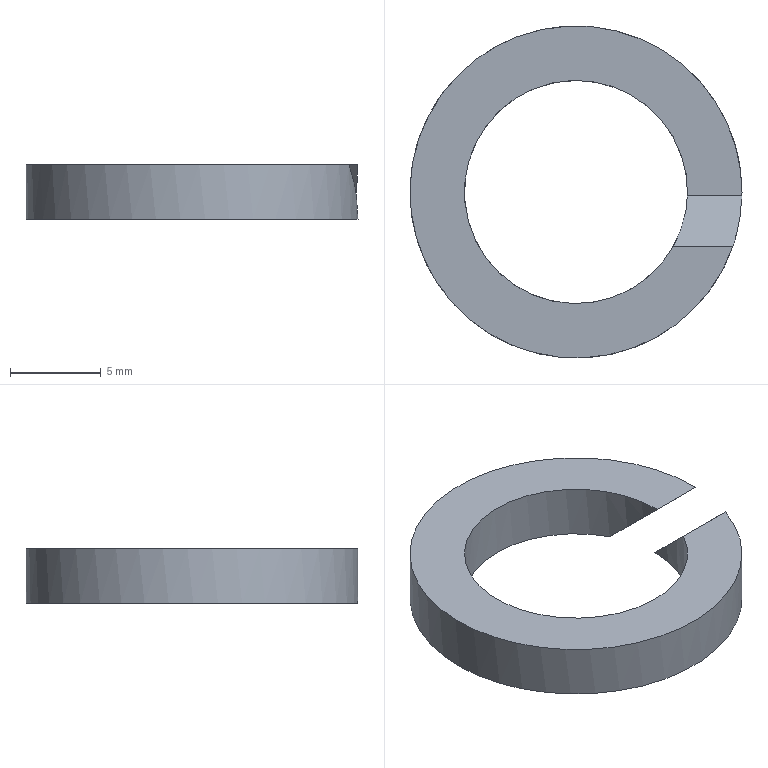Part | NX | features DATUM_CSYS 3, EXTRUDE 2, SKETCH 2 | 1 solid | 6 faces | box 18.3 x 18.3 x 3 mm | volume 406.803 mm3 | plane 4 | cylinder 2 | commonest cylinder face diameters 12.3 x1 18.3 x1
STEP:
#1=CARTESIAN_POINT('',(9.148,-0.1716,0.));
#2=VERTEX_POINT('',#1);
#3=CARTESIAN_POINT('',(8.644,-3.,0.));
#4=VERTEX_POINT('',#3);
#5=CARTESIAN_POINT('',(0.,0.,0.));
#6=DIRECTION('',(0.,0.,1.));
#7=DIRECTION('',(1.,0.,0.));
#8=AXIS2_PLACEMENT_3D('',#5,#6,#7);
#9=CIRCLE('',#8,9.15);
#10=EDGE_CURVE('',#2,#4,#9,.T.);
#11=ORIENTED_EDGE('',*,*,#10,.T.);
#12=CARTESIAN_POINT('',(5.369,-3.,0.));
#13=VERTEX_POINT('',#12);
#14=CARTESIAN_POINT('',(16.9,-3.,0.));
#15=DIRECTION('',(-1.,0.,0.));
#16=VECTOR('',#15,1000.);
#17=LINE('',#14,#16);
#18=EDGE_CURVE('',#4,#13,#17,.T.);
#19=ORIENTED_EDGE('',*,*,#18,.T.);
#20=CARTESIAN_POINT('',(6.148,-0.1716,0.));
#21=VERTEX_POINT('',#20);
#22=CARTESIAN_POINT('',(0.,0.,0.));
#23=DIRECTION('',(0.,0.,1.));
#24=DIRECTION('',(1.,0.,0.));
#25=AXIS2_PLACEMENT_3D('',#22,#23,#24);
#26=CIRCLE('',#25,6.15);
#27=EDGE_CURVE('',#21,#13,#26,.T.);
#28=ORIENTED_EDGE('',*,*,#27,.F.);
#29=CARTESIAN_POINT('',(16.9,-0.1716,0.));
#30=DIRECTION('',(-1.,0.,0.));
#31=VECTOR('',#30,1000.);
#32=LINE('',#29,#31);
#33=EDGE_CURVE('',#2,#21,#32,.T.);
#34=ORIENTED_EDGE('',*,*,#33,.F.);
#35=EDGE_LOOP('',(#11,#19,#28,#34));
#36=FACE_BOUND('',#35,.T.);
#37=CARTESIAN_POINT('',(0.,0.,0.));
#38=DIRECTION('',(0.,0.,1.));
#39=DIRECTION('',(1.,0.,0.));
#40=AXIS2_PLACEMENT_3D('',#37,#38,#39);
#41=PLANE('',#40);
#42=ADVANCED_FACE('',(#36),#41,.T.);
#43=CARTESIAN_POINT('',(8.702,2.828,-3.));
#44=VERTEX_POINT('',#43);
#45=CARTESIAN_POINT('',(0.,0.,-0.1716));
#46=DIRECTION('',(0.,0.7071,0.7071));
#47=DIRECTION('',(0.,-0.7071,0.7071));
#48=AXIS2_PLACEMENT_3D('',#45,#46,#47);
#49=ELLIPSE('',#48,12.94,9.15);
#50=EDGE_CURVE('',#44,#2,#49,.F.);
#51=ORIENTED_EDGE('',*,*,#50,.F.);
#52=CARTESIAN_POINT('',(9.15,0.,-3.));
#53=VERTEX_POINT('',#52);
#54=CARTESIAN_POINT('',(0.,0.,-3.));
#55=DIRECTION('',(0.,0.,1.));
#56=DIRECTION('',(1.,0.,0.));
#57=AXIS2_PLACEMENT_3D('',#54,#55,#56);
#58=CIRCLE('',#57,9.15);
#59=EDGE_CURVE('',#44,#53,#58,.T.);
#60=ORIENTED_EDGE('',*,*,#59,.T.);
#61=CARTESIAN_POINT('',(0.,0.,-3.));
#62=DIRECTION('',(0.,-0.7071,-0.7071));
#63=DIRECTION('',(0.,-0.7071,0.7071));
#64=AXIS2_PLACEMENT_3D('',#61,#62,#63);
#65=ELLIPSE('',#64,12.94,9.15);
#66=EDGE_CURVE('',#4,#53,#65,.F.);
#67=ORIENTED_EDGE('',*,*,#66,.F.);
#68=ORIENTED_EDGE('',*,*,#10,.F.);
#69=EDGE_LOOP('',(#51,#60,#67,#68));
#70=FACE_BOUND('',#69,.T.);
#71=CARTESIAN_POINT('',(0.,0.,-3.));
#72=DIRECTION('',(0.,0.,1.));
#73=DIRECTION('',(1.,0.,0.));
#74=AXIS2_PLACEMENT_3D('',#71,#72,#73);
#75=CYLINDRICAL_SURFACE('',#74,9.15);
#76=ADVANCED_FACE('',(#70),#75,.T.);
#77=CARTESIAN_POINT('',(5.461,2.828,-3.));
#78=VERTEX_POINT('',#77);
#79=CARTESIAN_POINT('',(6.15,0.,-3.));
#80=VERTEX_POINT('',#79);
#81=CARTESIAN_POINT('',(0.,0.,-3.));
#82=DIRECTION('',(0.,0.,1.));
#83=DIRECTION('',(1.,0.,0.));
#84=AXIS2_PLACEMENT_3D('',#81,#82,#83);
#85=CIRCLE('',#84,6.15);
#86=EDGE_CURVE('',#78,#80,#85,.T.);
#87=ORIENTED_EDGE('',*,*,#86,.F.);
#88=CARTESIAN_POINT('',(0.,0.,-0.1716));
#89=DIRECTION('',(0.,0.7071,0.7071));
#90=DIRECTION('',(0.,-0.7071,0.7071));
#91=AXIS2_PLACEMENT_3D('',#88,#89,#90);
#92=ELLIPSE('',#91,8.697,6.15);
#93=EDGE_CURVE('',#78,#21,#92,.F.);
#94=ORIENTED_EDGE('',*,*,#93,.T.);
#95=ORIENTED_EDGE('',*,*,#27,.T.);
#96=CARTESIAN_POINT('',(0.,0.,-3.));
#97=DIRECTION('',(0.,-0.7071,-0.7071));
#98=DIRECTION('',(0.,-0.7071,0.7071));
#99=AXIS2_PLACEMENT_3D('',#96,#97,#98);
#100=ELLIPSE('',#99,8.697,6.15);
#101=EDGE_CURVE('',#13,#80,#100,.F.);
#102=ORIENTED_EDGE('',*,*,#101,.T.);
#103=EDGE_LOOP('',(#87,#94,#95,#102));
#104=FACE_BOUND('',#103,.T.);
#105=CARTESIAN_POINT('',(0.,0.,-3.));
#106=DIRECTION('',(0.,0.,1.));
#107=DIRECTION('',(1.,0.,0.));
#108=AXIS2_PLACEMENT_3D('',#105,#106,#107);
#109=CYLINDRICAL_SURFACE('',#108,6.15);
#110=ADVANCED_FACE('',(#104),#109,.F.);
#111=ORIENTED_EDGE('',*,*,#59,.F.);
#112=CARTESIAN_POINT('',(16.9,2.828,-3.));
#113=DIRECTION('',(-1.,0.,0.));
#114=VECTOR('',#113,1000.);
#115=LINE('',#112,#114);
#116=EDGE_CURVE('',#44,#78,#115,.T.);
#117=ORIENTED_EDGE('',*,*,#116,.T.);
#118=ORIENTED_EDGE('',*,*,#86,.T.);
#119=CARTESIAN_POINT('',(16.9,0.,-3.));
#120=DIRECTION('',(-1.,0.,0.));
#121=VECTOR('',#120,1000.);
#122=LINE('',#119,#121);
#123=EDGE_CURVE('',#53,#80,#122,.T.);
#124=ORIENTED_EDGE('',*,*,#123,.F.);
#125=EDGE_LOOP('',(#111,#117,#118,#124));
#126=FACE_BOUND('',#125,.T.);
#127=CARTESIAN_POINT('',(0.,0.,-3.));
#128=DIRECTION('',(0.,0.,1.));
#129=DIRECTION('',(1.,0.,0.));
#130=AXIS2_PLACEMENT_3D('',#127,#128,#129);
#131=PLANE('',#130);
#132=ADVANCED_FACE('',(#126),#131,.F.);
#133=ORIENTED_EDGE('',*,*,#66,.T.);
#134=ORIENTED_EDGE('',*,*,#123,.T.);
#135=ORIENTED_EDGE('',*,*,#101,.F.);
#136=ORIENTED_EDGE('',*,*,#18,.F.);
#137=EDGE_LOOP('',(#133,#134,#135,#136));
#138=FACE_BOUND('',#137,.T.);
#139=CARTESIAN_POINT('',(16.9,0.,-3.));
#140=DIRECTION('',(0.,-0.7071,-0.7071));
#141=DIRECTION('',(0.,0.7071,-0.7071));
#142=AXIS2_PLACEMENT_3D('',#139,#140,#141);
#143=PLANE('',#142);
#144=ADVANCED_FACE('',(#138),#143,.F.);
#145=ORIENTED_EDGE('',*,*,#50,.T.);
#146=ORIENTED_EDGE('',*,*,#33,.T.);
#147=ORIENTED_EDGE('',*,*,#93,.F.);
#148=ORIENTED_EDGE('',*,*,#116,.F.);
#149=EDGE_LOOP('',(#145,#146,#147,#148));
#150=FACE_BOUND('',#149,.T.);
#151=CARTESIAN_POINT('',(16.9,-0.1716,0.));
#152=DIRECTION('',(0.,0.7071,0.7071));
#153=DIRECTION('',(0.,-0.7071,0.7071));
#154=AXIS2_PLACEMENT_3D('',#151,#152,#153);
#155=PLANE('',#154);
#156=ADVANCED_FACE('',(#150),#155,.F.);
#157=CLOSED_SHELL('',(#42,#76,#110,#132,#144,#156));
#158=MANIFOLD_SOLID_BREP('',#157);
#159=(LENGTH_UNIT()NAMED_UNIT(*)SI_UNIT(.MILLI.,.METRE.));
#160=UNCERTAINTY_MEASURE_WITH_UNIT(LENGTH_MEASURE(0.00001),#159,'','');
#161=(NAMED_UNIT(*)PLANE_ANGLE_UNIT()SI_UNIT($,.RADIAN.));
#162=(NAMED_UNIT(*)SI_UNIT($,.STERADIAN.)SOLID_ANGLE_UNIT());
#163=(GEOMETRIC_REPRESENTATION_CONTEXT(3)GLOBAL_UNCERTAINTY_ASSIGNED_CONTEXT((#160))GLOBAL_UNIT_ASSIGNED_CONTEXT((#159,#161,#162))REPRESENTATION_CONTEXT('',''));
#164=ADVANCED_BREP_SHAPE_REPRESENTATION('',(#158),#163);